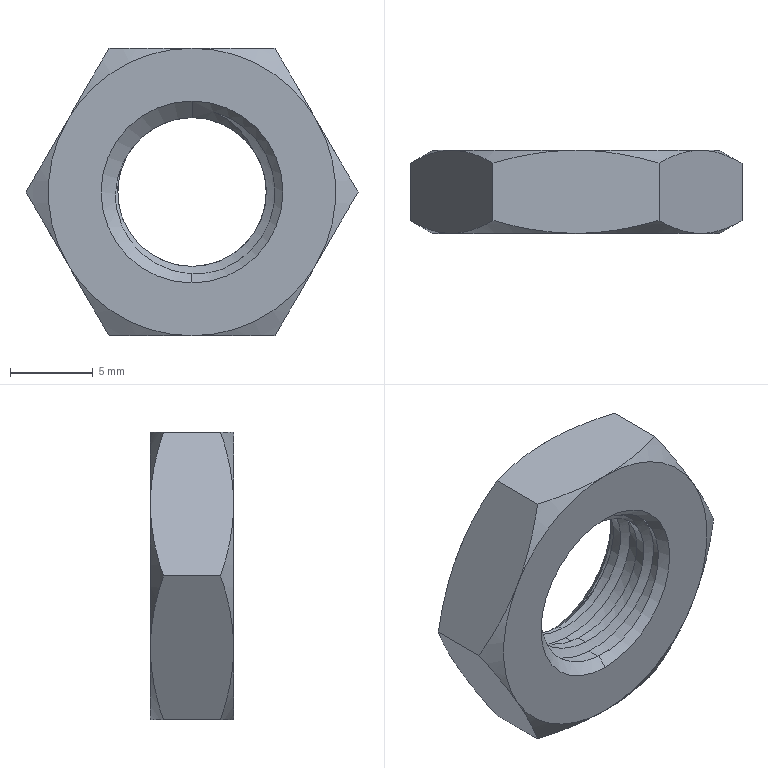Part | SolidWorks | features ICE 2, Chamfer 1, CombineBodies 1, Extrusion 1, MoveCopyBody 1, Stock 1 | 1 solid | 36 faces | box 20 x 5 x 17.321 mm | volume 912.864 mm3 | cone 16 | cylinder 10 | plane 8 | spline 2 | commonest cylinder face diameters 8.96 x5 10 x5